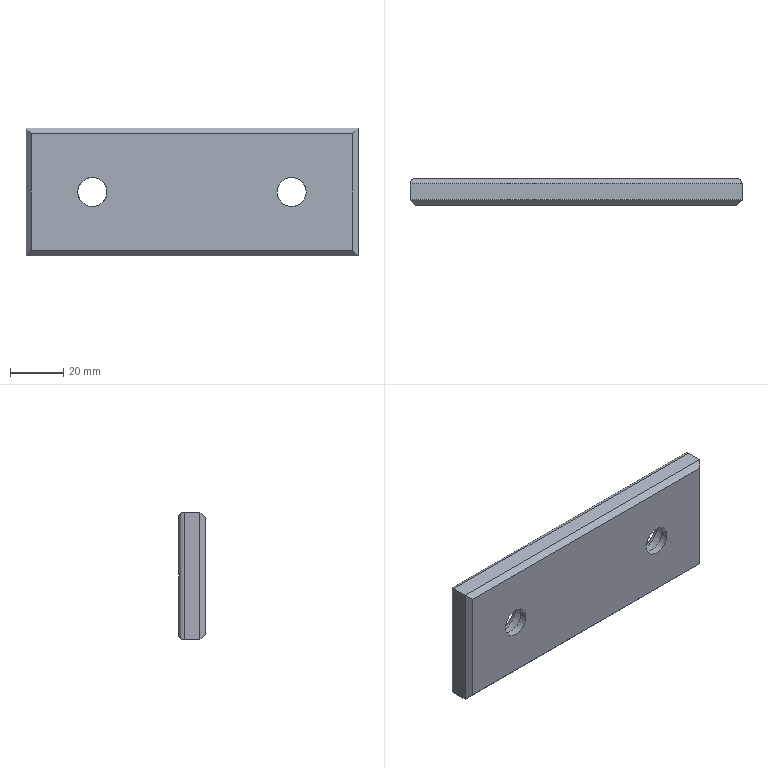Part | NX | features MAIN_BODY 2 | 1 solid | 22 faces | box 125 x 10 x 48 mm | volume 54901 mm3 | plane 12 | cylinder 8 | torus 2 | commonest cylinder face diameters 4 x4 11 x2 17.5 x2
STEP:
#1=CARTESIAN_POINT('',(-62.,230.,-137.));
#2=VERTEX_POINT('',#1);
#3=CARTESIAN_POINT('',(-183.,230.,-137.));
#4=VERTEX_POINT('',#3);
#5=CARTESIAN_POINT('',(-185.,230.,-137.));
#6=DIRECTION('',(1.,0.,0.));
#7=VECTOR('',#6,1000.);
#8=LINE('',#5,#7);
#9=EDGE_CURVE('',#2,#4,#8,.F.);
#10=ORIENTED_EDGE('',*,*,#9,.T.);
#11=CARTESIAN_POINT('',(-183.,230.,-93.));
#12=VERTEX_POINT('',#11);
#13=CARTESIAN_POINT('',(-183.,230.,-139.));
#14=DIRECTION('',(0.,0.,-1.));
#15=VECTOR('',#14,1000.);
#16=LINE('',#13,#15);
#17=EDGE_CURVE('',#4,#12,#16,.F.);
#18=ORIENTED_EDGE('',*,*,#17,.T.);
#19=CARTESIAN_POINT('',(-62.,230.,-93.));
#20=VERTEX_POINT('',#19);
#21=CARTESIAN_POINT('',(-185.,230.,-93.));
#22=DIRECTION('',(-1.,0.,0.));
#23=VECTOR('',#22,1000.);
#24=LINE('',#21,#23);
#25=EDGE_CURVE('',#12,#20,#24,.F.);
#26=ORIENTED_EDGE('',*,*,#25,.T.);
#27=CARTESIAN_POINT('',(-62.,230.,-139.));
#28=DIRECTION('',(0.,0.,1.));
#29=VECTOR('',#28,1000.);
#30=LINE('',#27,#29);
#31=EDGE_CURVE('',#20,#2,#30,.F.);
#32=ORIENTED_EDGE('',*,*,#31,.T.);
#33=EDGE_LOOP('',(#10,#18,#26,#32));
#34=FACE_BOUND('',#33,.T.);
#35=CARTESIAN_POINT('',(-170.75,230.,-115.));
#36=VERTEX_POINT('',#35);
#37=CARTESIAN_POINT('',(-160.,230.,-115.));
#38=DIRECTION('',(0.,1.,0.));
#39=DIRECTION('',(-1.,0.,0.));
#40=AXIS2_PLACEMENT_3D('',#37,#38,#39);
#41=CIRCLE('',#40,10.75);
#42=EDGE_CURVE('',#36,#36,#41,.F.);
#43=ORIENTED_EDGE('',*,*,#42,.T.);
#44=EDGE_LOOP('',(#43));
#45=FACE_BOUND('',#44,.T.);
#46=CARTESIAN_POINT('',(-95.75,230.,-115.));
#47=VERTEX_POINT('',#46);
#48=CARTESIAN_POINT('',(-85.,230.,-115.));
#49=DIRECTION('',(0.,1.,0.));
#50=DIRECTION('',(-1.,0.,0.));
#51=AXIS2_PLACEMENT_3D('',#48,#49,#50);
#52=CIRCLE('',#51,10.75);
#53=EDGE_CURVE('',#47,#47,#52,.F.);
#54=ORIENTED_EDGE('',*,*,#53,.T.);
#55=EDGE_LOOP('',(#54));
#56=FACE_BOUND('',#55,.T.);
#57=CARTESIAN_POINT('',(-185.,230.,-139.));
#58=DIRECTION('',(0.,1.,0.));
#59=DIRECTION('',(-1.,0.,0.));
#60=AXIS2_PLACEMENT_3D('',#57,#58,#59);
#61=PLANE('',#60);
#62=ADVANCED_FACE('',(#34,#45,#56),#61,.T.);
#63=CARTESIAN_POINT('',(-160.,220.,-109.5));
#64=VERTEX_POINT('',#63);
#65=CARTESIAN_POINT('',(-160.,220.,-115.));
#66=DIRECTION('',(0.,1.,0.));
#67=DIRECTION('',(0.,0.,1.));
#68=AXIS2_PLACEMENT_3D('',#65,#66,#67);
#69=CIRCLE('',#68,5.5);
#70=EDGE_CURVE('',#64,#64,#69,.T.);
#71=ORIENTED_EDGE('',*,*,#70,.F.);
#72=EDGE_LOOP('',(#71));
#73=FACE_BOUND('',#72,.T.);
#74=CARTESIAN_POINT('',(-165.5,222.7,-115.));
#75=VERTEX_POINT('',#74);
#76=CARTESIAN_POINT('',(-160.,222.7,-115.));
#77=DIRECTION('',(0.,1.,0.));
#78=DIRECTION('',(-1.,0.,0.));
#79=AXIS2_PLACEMENT_3D('',#76,#77,#78);
#80=CIRCLE('',#79,5.5);
#81=EDGE_CURVE('',#75,#75,#80,.T.);
#82=ORIENTED_EDGE('',*,*,#81,.T.);
#83=EDGE_LOOP('',(#82));
#84=FACE_BOUND('',#83,.T.);
#85=CARTESIAN_POINT('',(-160.,240.,-115.));
#86=DIRECTION('',(0.,-1.,0.));
#87=DIRECTION('',(1.,0.,0.));
#88=AXIS2_PLACEMENT_3D('',#85,#86,#87);
#89=CYLINDRICAL_SURFACE('',#88,5.5);
#90=ADVANCED_FACE('',(#73,#84),#89,.F.);
#91=CARTESIAN_POINT('',(-62.,220.,-93.));
#92=VERTEX_POINT('',#91);
#93=CARTESIAN_POINT('',(-183.,220.,-93.));
#94=VERTEX_POINT('',#93);
#95=CARTESIAN_POINT('',(-185.,220.,-93.));
#96=DIRECTION('',(-1.,0.,0.));
#97=VECTOR('',#96,1000.);
#98=LINE('',#95,#97);
#99=EDGE_CURVE('',#92,#94,#98,.T.);
#100=ORIENTED_EDGE('',*,*,#99,.T.);
#101=CARTESIAN_POINT('',(-183.,220.,-137.));
#102=VERTEX_POINT('',#101);
#103=CARTESIAN_POINT('',(-183.,220.,-139.));
#104=DIRECTION('',(0.,0.,-1.));
#105=VECTOR('',#104,1000.);
#106=LINE('',#103,#105);
#107=EDGE_CURVE('',#94,#102,#106,.T.);
#108=ORIENTED_EDGE('',*,*,#107,.T.);
#109=CARTESIAN_POINT('',(-62.,220.,-137.));
#110=VERTEX_POINT('',#109);
#111=CARTESIAN_POINT('',(-60.,220.,-137.));
#112=DIRECTION('',(1.,0.,0.));
#113=VECTOR('',#112,1000.);
#114=LINE('',#111,#113);
#115=EDGE_CURVE('',#102,#110,#114,.T.);
#116=ORIENTED_EDGE('',*,*,#115,.T.);
#117=CARTESIAN_POINT('',(-62.,220.,-91.));
#118=DIRECTION('',(0.,0.,1.));
#119=VECTOR('',#118,1000.);
#120=LINE('',#117,#119);
#121=EDGE_CURVE('',#110,#92,#120,.T.);
#122=ORIENTED_EDGE('',*,*,#121,.T.);
#123=EDGE_LOOP('',(#100,#108,#116,#122));
#124=FACE_BOUND('',#123,.T.);
#125=CARTESIAN_POINT('',(-85.,220.,-109.5));
#126=VERTEX_POINT('',#125);
#127=CARTESIAN_POINT('',(-85.,220.,-115.));
#128=DIRECTION('',(0.,-1.,0.));
#129=DIRECTION('',(0.,0.,1.));
#130=AXIS2_PLACEMENT_3D('',#127,#128,#129);
#131=CIRCLE('',#130,5.5);
#132=EDGE_CURVE('',#126,#126,#131,.T.);
#133=ORIENTED_EDGE('',*,*,#132,.F.);
#134=EDGE_LOOP('',(#133));
#135=FACE_BOUND('',#134,.T.);
#136=ORIENTED_EDGE('',*,*,#70,.T.);
#137=EDGE_LOOP('',(#136));
#138=FACE_BOUND('',#137,.T.);
#139=CARTESIAN_POINT('',(-185.,220.,-139.));
#140=DIRECTION('',(0.,1.,0.));
#141=DIRECTION('',(-1.,0.,0.));
#142=AXIS2_PLACEMENT_3D('',#139,#140,#141);
#143=PLANE('',#142);
#144=ADVANCED_FACE('',(#124,#135,#138),#143,.F.);
#145=CARTESIAN_POINT('',(-60.,228.,-139.));
#146=VERTEX_POINT('',#145);
#147=CARTESIAN_POINT('',(-60.,222.,-139.));
#148=VERTEX_POINT('',#147);
#149=CARTESIAN_POINT('',(-60.,230.,-139.));
#150=DIRECTION('',(0.,-1.,0.));
#151=VECTOR('',#150,1000.);
#152=LINE('',#149,#151);
#153=EDGE_CURVE('',#146,#148,#152,.T.);
#154=ORIENTED_EDGE('',*,*,#153,.T.);
#155=CARTESIAN_POINT('',(-185.,222.,-139.));
#156=VERTEX_POINT('',#155);
#157=CARTESIAN_POINT('',(-185.,222.,-139.));
#158=DIRECTION('',(-1.,0.,0.));
#159=VECTOR('',#158,1000.);
#160=LINE('',#157,#159);
#161=EDGE_CURVE('',#148,#156,#160,.T.);
#162=ORIENTED_EDGE('',*,*,#161,.T.);
#163=CARTESIAN_POINT('',(-185.,228.,-139.));
#164=VERTEX_POINT('',#163);
#165=CARTESIAN_POINT('',(-185.,230.,-139.));
#166=DIRECTION('',(0.,-1.,0.));
#167=VECTOR('',#166,1000.);
#168=LINE('',#165,#167);
#169=EDGE_CURVE('',#164,#156,#168,.T.);
#170=ORIENTED_EDGE('',*,*,#169,.F.);
#171=CARTESIAN_POINT('',(-185.,228.,-139.));
#172=DIRECTION('',(1.,0.,0.));
#173=VECTOR('',#172,1000.);
#174=LINE('',#171,#173);
#175=EDGE_CURVE('',#164,#146,#174,.T.);
#176=ORIENTED_EDGE('',*,*,#175,.T.);
#177=EDGE_LOOP('',(#154,#162,#170,#176));
#178=FACE_BOUND('',#177,.T.);
#179=CARTESIAN_POINT('',(-185.,230.,-139.));
#180=DIRECTION('',(0.,0.,-1.));
#181=DIRECTION('',(-1.,0.,0.));
#182=AXIS2_PLACEMENT_3D('',#179,#180,#181);
#183=PLANE('',#182);
#184=ADVANCED_FACE('',(#178),#183,.T.);
#185=CARTESIAN_POINT('',(-60.,228.,-91.));
#186=VERTEX_POINT('',#185);
#187=CARTESIAN_POINT('',(-60.,222.,-91.));
#188=VERTEX_POINT('',#187);
#189=CARTESIAN_POINT('',(-60.,230.,-91.));
#190=DIRECTION('',(0.,-1.,0.));
#191=VECTOR('',#190,1000.);
#192=LINE('',#189,#191);
#193=EDGE_CURVE('',#186,#188,#192,.T.);
#194=ORIENTED_EDGE('',*,*,#193,.T.);
#195=CARTESIAN_POINT('',(-60.,222.,-139.));
#196=DIRECTION('',(0.,0.,-1.));
#197=VECTOR('',#196,1000.);
#198=LINE('',#195,#197);
#199=EDGE_CURVE('',#188,#148,#198,.T.);
#200=ORIENTED_EDGE('',*,*,#199,.T.);
#201=ORIENTED_EDGE('',*,*,#153,.F.);
#202=CARTESIAN_POINT('',(-60.,228.,-139.));
#203=DIRECTION('',(0.,0.,1.));
#204=VECTOR('',#203,1000.);
#205=LINE('',#202,#204);
#206=EDGE_CURVE('',#146,#186,#205,.T.);
#207=ORIENTED_EDGE('',*,*,#206,.T.);
#208=EDGE_LOOP('',(#194,#200,#201,#207));
#209=FACE_BOUND('',#208,.T.);
#210=CARTESIAN_POINT('',(-60.,230.,-139.));
#211=DIRECTION('',(1.,0.,0.));
#212=DIRECTION('',(0.,1.,0.));
#213=AXIS2_PLACEMENT_3D('',#210,#211,#212);
#214=PLANE('',#213);
#215=ADVANCED_FACE('',(#209),#214,.T.);
#216=CARTESIAN_POINT('',(-185.,228.,-91.));
#217=VERTEX_POINT('',#216);
#218=CARTESIAN_POINT('',(-185.,222.,-91.));
#219=VERTEX_POINT('',#218);
#220=CARTESIAN_POINT('',(-185.,230.,-91.));
#221=DIRECTION('',(0.,-1.,0.));
#222=VECTOR('',#221,1000.);
#223=LINE('',#220,#222);
#224=EDGE_CURVE('',#217,#219,#223,.T.);
#225=ORIENTED_EDGE('',*,*,#224,.T.);
#226=CARTESIAN_POINT('',(-60.,222.,-91.));
#227=DIRECTION('',(1.,0.,0.));
#228=VECTOR('',#227,1000.);
#229=LINE('',#226,#228);
#230=EDGE_CURVE('',#219,#188,#229,.T.);
#231=ORIENTED_EDGE('',*,*,#230,.T.);
#232=ORIENTED_EDGE('',*,*,#193,.F.);
#233=CARTESIAN_POINT('',(-60.,228.,-91.));
#234=DIRECTION('',(-1.,0.,0.));
#235=VECTOR('',#234,1000.);
#236=LINE('',#233,#235);
#237=EDGE_CURVE('',#186,#217,#236,.T.);
#238=ORIENTED_EDGE('',*,*,#237,.T.);
#239=EDGE_LOOP('',(#225,#231,#232,#238));
#240=FACE_BOUND('',#239,.T.);
#241=CARTESIAN_POINT('',(-60.,230.,-91.));
#242=DIRECTION('',(0.,0.,1.));
#243=DIRECTION('',(1.,0.,0.));
#244=AXIS2_PLACEMENT_3D('',#241,#242,#243);
#245=PLANE('',#244);
#246=ADVANCED_FACE('',(#240),#245,.T.);
#247=ORIENTED_EDGE('',*,*,#169,.T.);
#248=CARTESIAN_POINT('',(-185.,222.,-91.));
#249=DIRECTION('',(0.,0.,1.));
#250=VECTOR('',#249,1000.);
#251=LINE('',#248,#250);
#252=EDGE_CURVE('',#156,#219,#251,.T.);
#253=ORIENTED_EDGE('',*,*,#252,.T.);
#254=ORIENTED_EDGE('',*,*,#224,.F.);
#255=CARTESIAN_POINT('',(-185.,228.,-91.));
#256=DIRECTION('',(0.,0.,-1.));
#257=VECTOR('',#256,1000.);
#258=LINE('',#255,#257);
#259=EDGE_CURVE('',#217,#164,#258,.T.);
#260=ORIENTED_EDGE('',*,*,#259,.T.);
#261=EDGE_LOOP('',(#247,#253,#254,#260));
#262=FACE_BOUND('',#261,.T.);
#263=CARTESIAN_POINT('',(-185.,230.,-91.));
#264=DIRECTION('',(-1.,0.,0.));
#265=DIRECTION('',(0.,0.,1.));
#266=AXIS2_PLACEMENT_3D('',#263,#264,#265);
#267=PLANE('',#266);
#268=ADVANCED_FACE('',(#262),#267,.T.);
#269=CARTESIAN_POINT('',(-79.5,222.7,-115.));
#270=VERTEX_POINT('',#269);
#271=CARTESIAN_POINT('',(-85.,222.7,-115.));
#272=DIRECTION('',(0.,-1.,0.));
#273=DIRECTION('',(1.,0.,0.));
#274=AXIS2_PLACEMENT_3D('',#271,#272,#273);
#275=CIRCLE('',#274,5.5);
#276=EDGE_CURVE('',#270,#270,#275,.F.);
#277=ORIENTED_EDGE('',*,*,#276,.T.);
#278=EDGE_LOOP('',(#277));
#279=FACE_BOUND('',#278,.T.);
#280=ORIENTED_EDGE('',*,*,#132,.T.);
#281=EDGE_LOOP('',(#280));
#282=FACE_BOUND('',#281,.T.);
#283=CARTESIAN_POINT('',(-85.,240.,-115.));
#284=DIRECTION('',(0.,-1.,0.));
#285=DIRECTION('',(1.,0.,0.));
#286=AXIS2_PLACEMENT_3D('',#283,#284,#285);
#287=CYLINDRICAL_SURFACE('',#286,5.5);
#288=ADVANCED_FACE('',(#279,#282),#287,.F.);
#289=CARTESIAN_POINT('',(-168.75,228.,-115.));
#290=VERTEX_POINT('',#289);
#291=CARTESIAN_POINT('',(-160.,228.,-115.));
#292=DIRECTION('',(0.,1.,0.));
#293=DIRECTION('',(-1.,0.,0.));
#294=AXIS2_PLACEMENT_3D('',#291,#292,#293);
#295=CIRCLE('',#294,8.75);
#296=EDGE_CURVE('',#290,#290,#295,.T.);
#297=ORIENTED_EDGE('',*,*,#296,.T.);
#298=EDGE_LOOP('',(#297));
#299=FACE_BOUND('',#298,.T.);
#300=CARTESIAN_POINT('',(-160.,222.7,-106.25));
#301=VERTEX_POINT('',#300);
#302=CARTESIAN_POINT('',(-160.,222.7,-115.));
#303=DIRECTION('',(0.,1.,0.));
#304=DIRECTION('',(0.,0.,1.));
#305=AXIS2_PLACEMENT_3D('',#302,#303,#304);
#306=CIRCLE('',#305,8.75);
#307=EDGE_CURVE('',#301,#301,#306,.T.);
#308=ORIENTED_EDGE('',*,*,#307,.F.);
#309=EDGE_LOOP('',(#308));
#310=FACE_BOUND('',#309,.T.);
#311=CARTESIAN_POINT('',(-160.,250.,-115.));
#312=DIRECTION('',(0.,-1.,0.));
#313=DIRECTION('',(1.,0.,0.));
#314=AXIS2_PLACEMENT_3D('',#311,#312,#313);
#315=CYLINDRICAL_SURFACE('',#314,8.75);
#316=ADVANCED_FACE('',(#299,#310),#315,.F.);
#317=ORIENTED_EDGE('',*,*,#81,.F.);
#318=EDGE_LOOP('',(#317));
#319=FACE_BOUND('',#318,.T.);
#320=ORIENTED_EDGE('',*,*,#307,.T.);
#321=EDGE_LOOP('',(#320));
#322=FACE_BOUND('',#321,.T.);
#323=CARTESIAN_POINT('',(-160.,222.7,-115.));
#324=DIRECTION('',(0.,1.,0.));
#325=DIRECTION('',(-1.,0.,0.));
#326=AXIS2_PLACEMENT_3D('',#323,#324,#325);
#327=PLANE('',#326);
#328=ADVANCED_FACE('',(#319,#322),#327,.T.);
#329=CARTESIAN_POINT('',(-85.,222.7,-106.25));
#330=VERTEX_POINT('',#329);
#331=CARTESIAN_POINT('',(-85.,222.7,-115.));
#332=DIRECTION('',(0.,-1.,0.));
#333=DIRECTION('',(0.,0.,1.));
#334=AXIS2_PLACEMENT_3D('',#331,#332,#333);
#335=CIRCLE('',#334,8.75);
#336=EDGE_CURVE('',#330,#330,#335,.T.);
#337=ORIENTED_EDGE('',*,*,#336,.F.);
#338=EDGE_LOOP('',(#337));
#339=FACE_BOUND('',#338,.T.);
#340=ORIENTED_EDGE('',*,*,#276,.F.);
#341=EDGE_LOOP('',(#340));
#342=FACE_BOUND('',#341,.T.);
#343=CARTESIAN_POINT('',(-85.,222.7,-115.));
#344=DIRECTION('',(0.,-1.,0.));
#345=DIRECTION('',(1.,0.,0.));
#346=AXIS2_PLACEMENT_3D('',#343,#344,#345);
#347=PLANE('',#346);
#348=ADVANCED_FACE('',(#339,#342),#347,.F.);
#349=CARTESIAN_POINT('',(-93.75,228.,-115.));
#350=VERTEX_POINT('',#349);
#351=CARTESIAN_POINT('',(-85.,228.,-115.));
#352=DIRECTION('',(0.,1.,0.));
#353=DIRECTION('',(-1.,0.,0.));
#354=AXIS2_PLACEMENT_3D('',#351,#352,#353);
#355=CIRCLE('',#354,8.75);
#356=EDGE_CURVE('',#350,#350,#355,.T.);
#357=ORIENTED_EDGE('',*,*,#356,.T.);
#358=EDGE_LOOP('',(#357));
#359=FACE_BOUND('',#358,.T.);
#360=ORIENTED_EDGE('',*,*,#336,.T.);
#361=EDGE_LOOP('',(#360));
#362=FACE_BOUND('',#361,.T.);
#363=CARTESIAN_POINT('',(-85.,250.,-115.));
#364=DIRECTION('',(0.,-1.,0.));
#365=DIRECTION('',(1.,0.,0.));
#366=AXIS2_PLACEMENT_3D('',#363,#364,#365);
#367=CYLINDRICAL_SURFACE('',#366,8.75);
#368=ADVANCED_FACE('',(#359,#362),#367,.F.);
#369=CARTESIAN_POINT('',(-62.,228.,-137.));
#370=DIRECTION('',(0.7071,0.,0.7071));
#371=DIRECTION('',(-0.7071,0.,0.7071));
#372=AXIS2_PLACEMENT_3D('',#369,#370,#371);
#373=ELLIPSE('',#372,2.828,2.);
#374=EDGE_CURVE('',#2,#146,#373,.F.);
#375=ORIENTED_EDGE('',*,*,#374,.F.);
#376=ORIENTED_EDGE('',*,*,#31,.F.);
#377=CARTESIAN_POINT('',(-62.,228.,-93.));
#378=DIRECTION('',(-0.7071,0.,0.7071));
#379=DIRECTION('',(0.7071,0.,0.7071));
#380=AXIS2_PLACEMENT_3D('',#377,#378,#379);
#381=ELLIPSE('',#380,2.828,2.);
#382=EDGE_CURVE('',#186,#20,#381,.T.);
#383=ORIENTED_EDGE('',*,*,#382,.F.);
#384=ORIENTED_EDGE('',*,*,#206,.F.);
#385=EDGE_LOOP('',(#375,#376,#383,#384));
#386=FACE_BOUND('',#385,.T.);
#387=CARTESIAN_POINT('',(-62.,228.,-139.));
#388=DIRECTION('',(0.,0.,1.));
#389=DIRECTION('',(1.,0.,0.));
#390=AXIS2_PLACEMENT_3D('',#387,#388,#389);
#391=CYLINDRICAL_SURFACE('',#390,2.);
#392=ADVANCED_FACE('',(#386),#391,.T.);
#393=ORIENTED_EDGE('',*,*,#382,.T.);
#394=ORIENTED_EDGE('',*,*,#25,.F.);
#395=CARTESIAN_POINT('',(-183.,228.,-93.));
#396=DIRECTION('',(-0.7071,0.,-0.7071));
#397=DIRECTION('',(-0.7071,0.,0.7071));
#398=AXIS2_PLACEMENT_3D('',#395,#396,#397);
#399=ELLIPSE('',#398,2.828,2.);
#400=EDGE_CURVE('',#217,#12,#399,.T.);
#401=ORIENTED_EDGE('',*,*,#400,.F.);
#402=ORIENTED_EDGE('',*,*,#237,.F.);
#403=EDGE_LOOP('',(#393,#394,#401,#402));
#404=FACE_BOUND('',#403,.T.);
#405=CARTESIAN_POINT('',(-60.,228.,-93.));
#406=DIRECTION('',(-1.,0.,0.));
#407=DIRECTION('',(0.,-1.,0.));
#408=AXIS2_PLACEMENT_3D('',#405,#406,#407);
#409=CYLINDRICAL_SURFACE('',#408,2.);
#410=ADVANCED_FACE('',(#404),#409,.T.);
#411=ORIENTED_EDGE('',*,*,#374,.T.);
#412=ORIENTED_EDGE('',*,*,#175,.F.);
#413=CARTESIAN_POINT('',(-183.,228.,-137.));
#414=DIRECTION('',(0.7071,0.,-0.7071));
#415=DIRECTION('',(0.7071,0.,0.7071));
#416=AXIS2_PLACEMENT_3D('',#413,#414,#415);
#417=ELLIPSE('',#416,2.828,2.);
#418=EDGE_CURVE('',#4,#164,#417,.F.);
#419=ORIENTED_EDGE('',*,*,#418,.F.);
#420=ORIENTED_EDGE('',*,*,#9,.F.);
#421=EDGE_LOOP('',(#411,#412,#419,#420));
#422=FACE_BOUND('',#421,.T.);
#423=CARTESIAN_POINT('',(-185.,228.,-137.));
#424=DIRECTION('',(1.,0.,0.));
#425=DIRECTION('',(0.,0.,-1.));
#426=AXIS2_PLACEMENT_3D('',#423,#424,#425);
#427=CYLINDRICAL_SURFACE('',#426,2.);
#428=ADVANCED_FACE('',(#422),#427,.T.);
#429=ORIENTED_EDGE('',*,*,#400,.T.);
#430=ORIENTED_EDGE('',*,*,#17,.F.);
#431=ORIENTED_EDGE('',*,*,#418,.T.);
#432=ORIENTED_EDGE('',*,*,#259,.F.);
#433=EDGE_LOOP('',(#429,#430,#431,#432));
#434=FACE_BOUND('',#433,.T.);
#435=CARTESIAN_POINT('',(-183.,228.,-91.));
#436=DIRECTION('',(0.,0.,-1.));
#437=DIRECTION('',(-1.,0.,0.));
#438=AXIS2_PLACEMENT_3D('',#435,#436,#437);
#439=CYLINDRICAL_SURFACE('',#438,2.);
#440=ADVANCED_FACE('',(#434),#439,.T.);
#441=ORIENTED_EDGE('',*,*,#296,.F.);
#442=EDGE_LOOP('',(#441));
#443=FACE_BOUND('',#442,.T.);
#444=ORIENTED_EDGE('',*,*,#42,.F.);
#445=EDGE_LOOP('',(#444));
#446=FACE_BOUND('',#445,.T.);
#447=CARTESIAN_POINT('',(-160.,228.,-115.));
#448=DIRECTION('',(0.,1.,0.));
#449=DIRECTION('',(-1.,0.,0.));
#450=AXIS2_PLACEMENT_3D('',#447,#448,#449);
#451=TOROIDAL_SURFACE('',#450,10.75,2.);
#452=ADVANCED_FACE('',(#443,#446),#451,.T.);
#453=ORIENTED_EDGE('',*,*,#53,.F.);
#454=EDGE_LOOP('',(#453));
#455=FACE_BOUND('',#454,.T.);
#456=ORIENTED_EDGE('',*,*,#356,.F.);
#457=EDGE_LOOP('',(#456));
#458=FACE_BOUND('',#457,.T.);
#459=CARTESIAN_POINT('',(-85.,228.,-115.));
#460=DIRECTION('',(0.,1.,0.));
#461=DIRECTION('',(-1.,0.,0.));
#462=AXIS2_PLACEMENT_3D('',#459,#460,#461);
#463=TOROIDAL_SURFACE('',#462,10.75,2.);
#464=ADVANCED_FACE('',(#455,#458),#463,.T.);
#465=CARTESIAN_POINT('',(-61.333,220.667,-137.667));
#466=DIRECTION('',(0.5774,0.5774,-0.5774));
#467=VECTOR('',#466,1000.);
#468=LINE('',#465,#467);
#469=EDGE_CURVE('',#148,#110,#468,.F.);
#470=ORIENTED_EDGE('',*,*,#469,.F.);
#471=ORIENTED_EDGE('',*,*,#199,.F.);
#472=CARTESIAN_POINT('',(-103.,179.,-134.));
#473=DIRECTION('',(0.5774,0.5774,0.5774));
#474=VECTOR('',#473,1000.);
#475=LINE('',#472,#474);
#476=EDGE_CURVE('',#92,#188,#475,.T.);
#477=ORIENTED_EDGE('',*,*,#476,.F.);
#478=ORIENTED_EDGE('',*,*,#121,.F.);
#479=EDGE_LOOP('',(#470,#471,#477,#478));
#480=FACE_BOUND('',#479,.T.);
#481=CARTESIAN_POINT('',(-62.,220.,-139.));
#482=DIRECTION('',(0.7071,-0.7071,0.));
#483=DIRECTION('',(0.7071,0.7071,0.));
#484=AXIS2_PLACEMENT_3D('',#481,#482,#483);
#485=PLANE('',#484);
#486=ADVANCED_FACE('',(#480),#485,.T.);
#487=ORIENTED_EDGE('',*,*,#476,.T.);
#488=ORIENTED_EDGE('',*,*,#230,.F.);
#489=CARTESIAN_POINT('',(-183.667,220.667,-92.333));
#490=DIRECTION('',(0.5774,-0.5774,-0.5774));
#491=VECTOR('',#490,1000.);
#492=LINE('',#489,#491);
#493=EDGE_CURVE('',#94,#219,#492,.F.);
#494=ORIENTED_EDGE('',*,*,#493,.F.);
#495=ORIENTED_EDGE('',*,*,#99,.F.);
#496=EDGE_LOOP('',(#487,#488,#494,#495));
#497=FACE_BOUND('',#496,.T.);
#498=CARTESIAN_POINT('',(-185.,220.,-93.));
#499=DIRECTION('',(0.,-0.7071,0.7071));
#500=DIRECTION('',(0.,-0.7071,-0.7071));
#501=AXIS2_PLACEMENT_3D('',#498,#499,#500);
#502=PLANE('',#501);
#503=ADVANCED_FACE('',(#497),#502,.T.);
#504=ORIENTED_EDGE('',*,*,#469,.T.);
#505=ORIENTED_EDGE('',*,*,#115,.F.);
#506=CARTESIAN_POINT('',(-183.667,220.667,-137.667));
#507=DIRECTION('',(-0.5774,0.5774,-0.5774));
#508=VECTOR('',#507,1000.);
#509=LINE('',#506,#508);
#510=EDGE_CURVE('',#156,#102,#509,.F.);
#511=ORIENTED_EDGE('',*,*,#510,.F.);
#512=ORIENTED_EDGE('',*,*,#161,.F.);
#513=EDGE_LOOP('',(#504,#505,#511,#512));
#514=FACE_BOUND('',#513,.T.);
#515=CARTESIAN_POINT('',(-185.,220.,-137.));
#516=DIRECTION('',(0.,-0.7071,-0.7071));
#517=DIRECTION('',(0.,0.7071,-0.7071));
#518=AXIS2_PLACEMENT_3D('',#515,#516,#517);
#519=PLANE('',#518);
#520=ADVANCED_FACE('',(#514),#519,.T.);
#521=ORIENTED_EDGE('',*,*,#493,.T.);
#522=ORIENTED_EDGE('',*,*,#252,.F.);
#523=ORIENTED_EDGE('',*,*,#510,.T.);
#524=ORIENTED_EDGE('',*,*,#107,.F.);
#525=EDGE_LOOP('',(#521,#522,#523,#524));
#526=FACE_BOUND('',#525,.T.);
#527=CARTESIAN_POINT('',(-183.,220.,-139.));
#528=DIRECTION('',(-0.7071,-0.7071,0.));
#529=DIRECTION('',(0.7071,-0.7071,0.));
#530=AXIS2_PLACEMENT_3D('',#527,#528,#529);
#531=PLANE('',#530);
#532=ADVANCED_FACE('',(#526),#531,.T.);
#533=CLOSED_SHELL('',(#62,#90,#144,#184,#215,#246,#268,#288,#316,#328,#348,#368,#392,#410,#428,#440,#452,#464,#486,#503,#520,#532));
#534=MANIFOLD_SOLID_BREP('',#533);
#535=(LENGTH_UNIT()NAMED_UNIT(*)SI_UNIT(.MILLI.,.METRE.));
#536=UNCERTAINTY_MEASURE_WITH_UNIT(LENGTH_MEASURE(0.00001),#535,'','');
#537=(NAMED_UNIT(*)PLANE_ANGLE_UNIT()SI_UNIT($,.RADIAN.));
#538=(NAMED_UNIT(*)SI_UNIT($,.STERADIAN.)SOLID_ANGLE_UNIT());
#539=(GEOMETRIC_REPRESENTATION_CONTEXT(3)GLOBAL_UNCERTAINTY_ASSIGNED_CONTEXT((#536))GLOBAL_UNIT_ASSIGNED_CONTEXT((#535,#537,#538))REPRESENTATION_CONTEXT('',''));
#540=ADVANCED_BREP_SHAPE_REPRESENTATION('',(#534),#539);